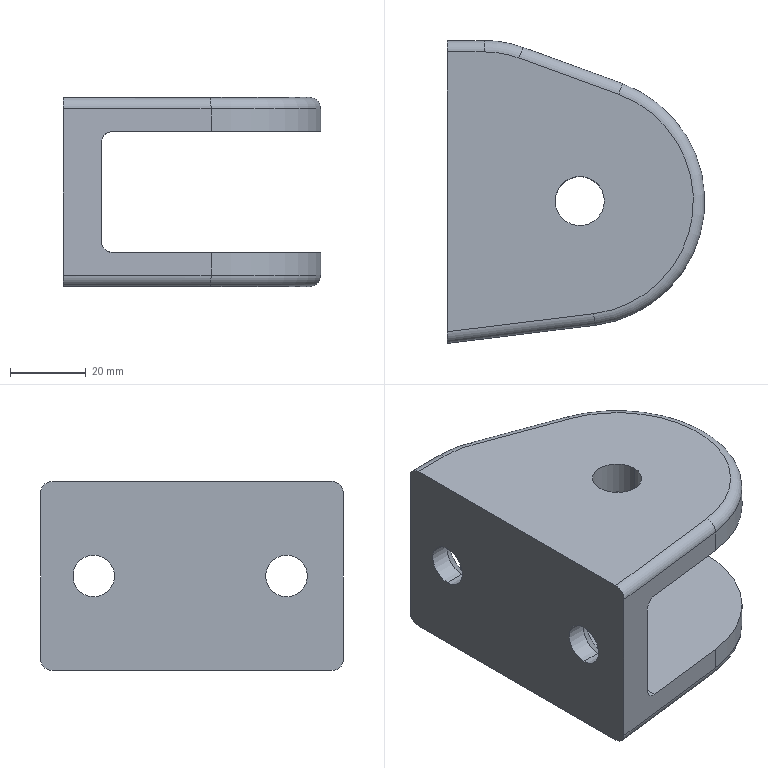Part | SolidWorks | features Fillet 2, ICE 2, Extrusion 1, HoleWzd 1 | 1 solid | 37 faces | box 68.028 x 80 x 50 mm | volume 98491 mm3 | cylinder 19 | plane 10 | cone 4 | torus 4 | commonest cylinder face diameters 6 x8 11 x4 13 x4 66.055 x2 60 x1
STEP:
#1=CARTESIAN_POINT('',(5.35,65.999,5.5));
#2=VERTEX_POINT('',#1);
#3=CARTESIAN_POINT('',(5.35,65.999,-5.5));
#4=VERTEX_POINT('',#3);
#5=CARTESIAN_POINT('',(5.35,65.999,0.));
#6=DIRECTION('',(1.,0.,0.));
#7=DIRECTION('',(0.,0.,-1.));
#8=AXIS2_PLACEMENT_3D('',#5,#6,#7);
#9=CIRCLE('',#8,5.5);
#10=EDGE_CURVE('',#2,#4,#9,.T.);
#11=ORIENTED_EDGE('',*,*,#10,.F.);
#12=CARTESIAN_POINT('',(10.,65.999,10.15));
#13=VERTEX_POINT('',#12);
#14=CARTESIAN_POINT('',(10.,65.999,10.15));
#15=DIRECTION('',(0.7071,0.,0.7071));
#16=VECTOR('',#15,1000.);
#17=LINE('',#14,#16);
#18=EDGE_CURVE('',#2,#13,#17,.T.);
#19=ORIENTED_EDGE('',*,*,#18,.T.);
#20=CARTESIAN_POINT('',(10.,65.999,-10.15));
#21=VERTEX_POINT('',#20);
#22=CARTESIAN_POINT('',(10.,65.999,0.));
#23=DIRECTION('',(1.,0.,0.));
#24=DIRECTION('',(0.,0.,-1.));
#25=AXIS2_PLACEMENT_3D('',#22,#23,#24);
#26=CIRCLE('',#25,10.15);
#27=EDGE_CURVE('',#13,#21,#26,.T.);
#28=ORIENTED_EDGE('',*,*,#27,.T.);
#29=CARTESIAN_POINT('',(10.,65.999,-10.15));
#30=DIRECTION('',(0.7071,0.,-0.7071));
#31=VECTOR('',#30,1000.);
#32=LINE('',#29,#31);
#33=EDGE_CURVE('',#4,#21,#32,.T.);
#34=ORIENTED_EDGE('',*,*,#33,.F.);
#35=EDGE_LOOP('',(#11,#19,#28,#34));
#36=FACE_OUTER_BOUND('',#35,.T.);
#37=CARTESIAN_POINT('',(10.,65.999,0.));
#38=DIRECTION('',(1.,0.,0.));
#39=DIRECTION('',(0.,0.,-1.));
#40=AXIS2_PLACEMENT_3D('',#37,#38,#39);
#41=CONICAL_SURFACE('',#40,10.15,0.7854);
#42=ADVANCED_FACE('',(#36),#41,.F.);
#43=CARTESIAN_POINT('',(0.,65.999,5.5));
#44=VERTEX_POINT('',#43);
#45=CARTESIAN_POINT('',(0.,65.999,-5.5));
#46=VERTEX_POINT('',#45);
#47=CARTESIAN_POINT('',(0.,65.999,0.));
#48=DIRECTION('',(1.,0.,0.));
#49=DIRECTION('',(0.,0.,-1.));
#50=AXIS2_PLACEMENT_3D('',#47,#48,#49);
#51=CIRCLE('',#50,5.5);
#52=EDGE_CURVE('',#44,#46,#51,.T.);
#53=ORIENTED_EDGE('',*,*,#52,.F.);
#54=CARTESIAN_POINT('',(10.,65.999,5.5));
#55=DIRECTION('',(1.,0.,0.));
#56=VECTOR('',#55,1000.);
#57=LINE('',#54,#56);
#58=EDGE_CURVE('',#44,#2,#57,.T.);
#59=ORIENTED_EDGE('',*,*,#58,.T.);
#60=ORIENTED_EDGE('',*,*,#10,.T.);
#61=CARTESIAN_POINT('',(10.,65.999,-5.5));
#62=DIRECTION('',(1.,0.,0.));
#63=VECTOR('',#62,1000.);
#64=LINE('',#61,#63);
#65=EDGE_CURVE('',#46,#4,#64,.T.);
#66=ORIENTED_EDGE('',*,*,#65,.F.);
#67=EDGE_LOOP('',(#53,#59,#60,#66));
#68=FACE_OUTER_BOUND('',#67,.T.);
#69=CARTESIAN_POINT('',(10.,65.999,0.));
#70=DIRECTION('',(1.,0.,0.));
#71=DIRECTION('',(0.,0.,-1.));
#72=AXIS2_PLACEMENT_3D('',#69,#70,#71);
#73=CYLINDRICAL_SURFACE('',#72,5.5);
#74=ADVANCED_FACE('',(#68),#73,.F.);
#75=CARTESIAN_POINT('',(5.35,15.,5.5));
#76=VERTEX_POINT('',#75);
#77=CARTESIAN_POINT('',(5.35,15.,-5.5));
#78=VERTEX_POINT('',#77);
#79=CARTESIAN_POINT('',(5.35,15.,0.));
#80=DIRECTION('',(1.,0.,0.));
#81=DIRECTION('',(0.,0.,-1.));
#82=AXIS2_PLACEMENT_3D('',#79,#80,#81);
#83=CIRCLE('',#82,5.5);
#84=EDGE_CURVE('',#76,#78,#83,.T.);
#85=ORIENTED_EDGE('',*,*,#84,.F.);
#86=CARTESIAN_POINT('',(10.,15.,10.15));
#87=VERTEX_POINT('',#86);
#88=CARTESIAN_POINT('',(10.,15.,10.15));
#89=DIRECTION('',(0.7071,0.,0.7071));
#90=VECTOR('',#89,1000.);
#91=LINE('',#88,#90);
#92=EDGE_CURVE('',#76,#87,#91,.T.);
#93=ORIENTED_EDGE('',*,*,#92,.T.);
#94=CARTESIAN_POINT('',(10.,15.,-10.15));
#95=VERTEX_POINT('',#94);
#96=CARTESIAN_POINT('',(10.,15.,0.));
#97=DIRECTION('',(1.,0.,0.));
#98=DIRECTION('',(0.,0.,-1.));
#99=AXIS2_PLACEMENT_3D('',#96,#97,#98);
#100=CIRCLE('',#99,10.15);
#101=EDGE_CURVE('',#87,#95,#100,.T.);
#102=ORIENTED_EDGE('',*,*,#101,.T.);
#103=CARTESIAN_POINT('',(10.,15.,-10.15));
#104=DIRECTION('',(0.7071,0.,-0.7071));
#105=VECTOR('',#104,1000.);
#106=LINE('',#103,#105);
#107=EDGE_CURVE('',#78,#95,#106,.T.);
#108=ORIENTED_EDGE('',*,*,#107,.F.);
#109=EDGE_LOOP('',(#85,#93,#102,#108));
#110=FACE_OUTER_BOUND('',#109,.T.);
#111=CARTESIAN_POINT('',(10.,15.,0.));
#112=DIRECTION('',(1.,0.,0.));
#113=DIRECTION('',(0.,0.,-1.));
#114=AXIS2_PLACEMENT_3D('',#111,#112,#113);
#115=CONICAL_SURFACE('',#114,10.15,0.7854);
#116=ADVANCED_FACE('',(#110),#115,.F.);
#117=CARTESIAN_POINT('',(0.,15.,5.5));
#118=VERTEX_POINT('',#117);
#119=CARTESIAN_POINT('',(0.,15.,-5.5));
#120=VERTEX_POINT('',#119);
#121=CARTESIAN_POINT('',(0.,15.,0.));
#122=DIRECTION('',(1.,0.,0.));
#123=DIRECTION('',(0.,0.,-1.));
#124=AXIS2_PLACEMENT_3D('',#121,#122,#123);
#125=CIRCLE('',#124,5.5);
#126=EDGE_CURVE('',#118,#120,#125,.T.);
#127=ORIENTED_EDGE('',*,*,#126,.F.);
#128=CARTESIAN_POINT('',(10.,15.,5.5));
#129=DIRECTION('',(1.,0.,0.));
#130=VECTOR('',#129,1000.);
#131=LINE('',#128,#130);
#132=EDGE_CURVE('',#118,#76,#131,.T.);
#133=ORIENTED_EDGE('',*,*,#132,.T.);
#134=ORIENTED_EDGE('',*,*,#84,.T.);
#135=CARTESIAN_POINT('',(10.,15.,-5.5));
#136=DIRECTION('',(1.,0.,0.));
#137=VECTOR('',#136,1000.);
#138=LINE('',#135,#137);
#139=EDGE_CURVE('',#120,#78,#138,.T.);
#140=ORIENTED_EDGE('',*,*,#139,.F.);
#141=EDGE_LOOP('',(#127,#133,#134,#140));
#142=FACE_OUTER_BOUND('',#141,.T.);
#143=CARTESIAN_POINT('',(10.,15.,0.));
#144=DIRECTION('',(1.,0.,0.));
#145=DIRECTION('',(0.,0.,-1.));
#146=AXIS2_PLACEMENT_3D('',#143,#144,#145);
#147=CYLINDRICAL_SURFACE('',#146,5.5);
#148=ADVANCED_FACE('',(#142),#147,.F.);
#149=CARTESIAN_POINT('',(28.5,37.573,-25.));
#150=VERTEX_POINT('',#149);
#151=CARTESIAN_POINT('',(41.5,37.573,-25.));
#152=VERTEX_POINT('',#151);
#153=CARTESIAN_POINT('',(35.,37.573,-25.));
#154=DIRECTION('',(0.,0.,1.));
#155=DIRECTION('',(1.,0.,0.));
#156=AXIS2_PLACEMENT_3D('',#153,#154,#155);
#157=CIRCLE('',#156,6.5);
#158=EDGE_CURVE('',#150,#152,#157,.T.);
#159=ORIENTED_EDGE('',*,*,#158,.F.);
#160=CARTESIAN_POINT('',(28.5,37.573,-16.));
#161=VERTEX_POINT('',#160);
#162=CARTESIAN_POINT('',(28.5,37.573,-25.));
#163=DIRECTION('',(0.,0.,1.));
#164=VECTOR('',#163,1000.);
#165=LINE('',#162,#164);
#166=EDGE_CURVE('',#150,#161,#165,.T.);
#167=ORIENTED_EDGE('',*,*,#166,.T.);
#168=CARTESIAN_POINT('',(41.5,37.573,-16.));
#169=VERTEX_POINT('',#168);
#170=CARTESIAN_POINT('',(35.,37.573,-16.));
#171=DIRECTION('',(0.,0.,1.));
#172=DIRECTION('',(1.,0.,0.));
#173=AXIS2_PLACEMENT_3D('',#170,#171,#172);
#174=CIRCLE('',#173,6.5);
#175=EDGE_CURVE('',#161,#169,#174,.T.);
#176=ORIENTED_EDGE('',*,*,#175,.T.);
#177=CARTESIAN_POINT('',(41.5,37.573,-25.));
#178=DIRECTION('',(0.,0.,1.));
#179=VECTOR('',#178,1000.);
#180=LINE('',#177,#179);
#181=EDGE_CURVE('',#152,#169,#180,.T.);
#182=ORIENTED_EDGE('',*,*,#181,.F.);
#183=EDGE_LOOP('',(#159,#167,#176,#182));
#184=FACE_OUTER_BOUND('',#183,.T.);
#185=CARTESIAN_POINT('',(35.,37.573,-25.));
#186=DIRECTION('',(0.,0.,1.));
#187=DIRECTION('',(1.,0.,0.));
#188=AXIS2_PLACEMENT_3D('',#185,#186,#187);
#189=CYLINDRICAL_SURFACE('',#188,6.5);
#190=ADVANCED_FACE('',(#184),#189,.F.);
#191=CARTESIAN_POINT('',(28.5,37.573,16.));
#192=VERTEX_POINT('',#191);
#193=CARTESIAN_POINT('',(41.5,37.573,16.));
#194=VERTEX_POINT('',#193);
#195=CARTESIAN_POINT('',(35.,37.573,16.));
#196=DIRECTION('',(0.,0.,1.));
#197=DIRECTION('',(1.,0.,0.));
#198=AXIS2_PLACEMENT_3D('',#195,#196,#197);
#199=CIRCLE('',#198,6.5);
#200=EDGE_CURVE('',#192,#194,#199,.T.);
#201=ORIENTED_EDGE('',*,*,#200,.F.);
#202=CARTESIAN_POINT('',(28.5,37.573,25.));
#203=VERTEX_POINT('',#202);
#204=CARTESIAN_POINT('',(28.5,37.573,-25.));
#205=DIRECTION('',(0.,0.,1.));
#206=VECTOR('',#205,1000.);
#207=LINE('',#204,#206);
#208=EDGE_CURVE('',#192,#203,#207,.T.);
#209=ORIENTED_EDGE('',*,*,#208,.T.);
#210=CARTESIAN_POINT('',(41.5,37.573,25.));
#211=VERTEX_POINT('',#210);
#212=CARTESIAN_POINT('',(35.,37.573,25.));
#213=DIRECTION('',(0.,0.,1.));
#214=DIRECTION('',(1.,0.,0.));
#215=AXIS2_PLACEMENT_3D('',#212,#213,#214);
#216=CIRCLE('',#215,6.5);
#217=EDGE_CURVE('',#203,#211,#216,.T.);
#218=ORIENTED_EDGE('',*,*,#217,.T.);
#219=CARTESIAN_POINT('',(41.5,37.573,-25.));
#220=DIRECTION('',(0.,0.,1.));
#221=VECTOR('',#220,1000.);
#222=LINE('',#219,#221);
#223=EDGE_CURVE('',#194,#211,#222,.T.);
#224=ORIENTED_EDGE('',*,*,#223,.F.);
#225=EDGE_LOOP('',(#201,#209,#218,#224));
#226=FACE_OUTER_BOUND('',#225,.T.);
#227=CARTESIAN_POINT('',(35.,37.573,-25.));
#228=DIRECTION('',(0.,0.,1.));
#229=DIRECTION('',(1.,0.,0.));
#230=AXIS2_PLACEMENT_3D('',#227,#228,#229);
#231=CYLINDRICAL_SURFACE('',#230,6.5);
#232=ADVANCED_FACE('',(#226),#231,.F.);
#233=CARTESIAN_POINT('',(0.,0.,22.));
#234=VERTEX_POINT('',#233);
#235=CARTESIAN_POINT('',(0.,0.,-22.));
#236=VERTEX_POINT('',#235);
#237=CARTESIAN_POINT('',(0.,0.,25.));
#238=DIRECTION('',(0.,0.,-1.));
#239=VECTOR('',#238,1000.);
#240=LINE('',#237,#239);
#241=EDGE_CURVE('',#234,#236,#240,.T.);
#242=ORIENTED_EDGE('',*,*,#241,.T.);
#243=CARTESIAN_POINT('',(39.025,4.792,-22.));
#244=VERTEX_POINT('',#243);
#245=CARTESIAN_POINT('',(39.025,4.792,-22.));
#246=DIRECTION('',(0.9925,0.1219,0.));
#247=VECTOR('',#246,1000.);
#248=LINE('',#245,#247);
#249=EDGE_CURVE('',#236,#244,#248,.T.);
#250=ORIENTED_EDGE('',*,*,#249,.T.);
#251=CARTESIAN_POINT('',(39.025,4.792,-16.));
#252=VERTEX_POINT('',#251);
#253=CARTESIAN_POINT('',(39.025,4.792,25.));
#254=DIRECTION('',(0.,0.,-1.));
#255=VECTOR('',#254,1000.);
#256=LINE('',#253,#255);
#257=EDGE_CURVE('',#252,#244,#256,.T.);
#258=ORIENTED_EDGE('',*,*,#257,.F.);
#259=CARTESIAN_POINT('',(13.,1.596,-16.));
#260=VERTEX_POINT('',#259);
#261=CARTESIAN_POINT('',(39.025,4.792,-16.));
#262=DIRECTION('',(0.9925,0.1219,0.));
#263=VECTOR('',#262,1000.);
#264=LINE('',#261,#263);
#265=EDGE_CURVE('',#260,#252,#264,.T.);
#266=ORIENTED_EDGE('',*,*,#265,.F.);
#267=CARTESIAN_POINT('',(10.,1.228,-13.));
#268=VERTEX_POINT('',#267);
#269=CARTESIAN_POINT('',(13.,1.596,-16.));
#270=CARTESIAN_POINT('',(11.243,1.38,-16.));
#271=CARTESIAN_POINT('',(10.,1.228,-14.757));
#272=CARTESIAN_POINT('',(10.,1.228,-13.));
#273=(BOUNDED_CURVE()B_SPLINE_CURVE(3,(#269,#270,#271,#272),.UNSPECIFIED.,.F.,.F.)B_SPLINE_CURVE_WITH_KNOTS((4,4),(4.712,6.283),.UNSPECIFIED.)CURVE()GEOMETRIC_REPRESENTATION_ITEM()RATIONAL_B_SPLINE_CURVE((1.,0.8047,0.8047,1.))REPRESENTATION_ITEM(''));
#274=EDGE_CURVE('',#260,#268,#273,.T.);
#275=ORIENTED_EDGE('',*,*,#274,.T.);
#276=CARTESIAN_POINT('',(10.,1.228,13.));
#277=VERTEX_POINT('',#276);
#278=CARTESIAN_POINT('',(10.,1.228,25.));
#279=DIRECTION('',(0.,0.,1.));
#280=VECTOR('',#279,1000.);
#281=LINE('',#278,#280);
#282=EDGE_CURVE('',#268,#277,#281,.T.);
#283=ORIENTED_EDGE('',*,*,#282,.T.);
#284=CARTESIAN_POINT('',(13.,1.596,16.));
#285=VERTEX_POINT('',#284);
#286=CARTESIAN_POINT('',(10.,1.228,13.));
#287=CARTESIAN_POINT('',(10.,1.228,14.757));
#288=CARTESIAN_POINT('',(11.243,1.38,16.));
#289=CARTESIAN_POINT('',(13.,1.596,16.));
#290=(BOUNDED_CURVE()B_SPLINE_CURVE(3,(#286,#287,#288,#289),.UNSPECIFIED.,.F.,.F.)B_SPLINE_CURVE_WITH_KNOTS((4,4),(3.142,4.712),.UNSPECIFIED.)CURVE()GEOMETRIC_REPRESENTATION_ITEM()RATIONAL_B_SPLINE_CURVE((1.,0.8047,0.8047,1.))REPRESENTATION_ITEM(''));
#291=EDGE_CURVE('',#277,#285,#290,.T.);
#292=ORIENTED_EDGE('',*,*,#291,.T.);
#293=CARTESIAN_POINT('',(39.025,4.792,16.));
#294=VERTEX_POINT('',#293);
#295=CARTESIAN_POINT('',(39.025,4.792,16.));
#296=DIRECTION('',(0.9925,0.1219,0.));
#297=VECTOR('',#296,1000.);
#298=LINE('',#295,#297);
#299=EDGE_CURVE('',#285,#294,#298,.T.);
#300=ORIENTED_EDGE('',*,*,#299,.T.);
#301=CARTESIAN_POINT('',(39.025,4.792,22.));
#302=VERTEX_POINT('',#301);
#303=CARTESIAN_POINT('',(39.025,4.792,25.));
#304=DIRECTION('',(0.,0.,-1.));
#305=VECTOR('',#304,1000.);
#306=LINE('',#303,#305);
#307=EDGE_CURVE('',#302,#294,#306,.T.);
#308=ORIENTED_EDGE('',*,*,#307,.F.);
#309=CARTESIAN_POINT('',(39.025,4.792,22.));
#310=DIRECTION('',(-0.9925,-0.1219,0.));
#311=VECTOR('',#310,1000.);
#312=LINE('',#309,#311);
#313=EDGE_CURVE('',#302,#234,#312,.T.);
#314=ORIENTED_EDGE('',*,*,#313,.T.);
#315=EDGE_LOOP('',(#242,#250,#258,#266,#275,#283,#292,#300,#308,#314));
#316=FACE_OUTER_BOUND('',#315,.T.);
#317=CARTESIAN_POINT('',(39.025,4.792,25.));
#318=DIRECTION('',(-0.1219,0.9925,0.));
#319=DIRECTION('',(-0.9925,-0.1219,0.));
#320=AXIS2_PLACEMENT_3D('',#317,#318,#319);
#321=PLANE('',#320);
#322=ADVANCED_FACE('',(#316),#321,.F.);
#323=ORIENTED_EDGE('',*,*,#257,.T.);
#324=CARTESIAN_POINT('',(46.296,68.609,-22.));
#325=VERTEX_POINT('',#324);
#326=CARTESIAN_POINT('',(35.,37.573,-22.));
#327=DIRECTION('',(0.,0.,1.));
#328=DIRECTION('',(-1.,0.,0.));
#329=AXIS2_PLACEMENT_3D('',#326,#327,#328);
#330=CIRCLE('',#329,33.028);
#331=EDGE_CURVE('',#244,#325,#330,.T.);
#332=ORIENTED_EDGE('',*,*,#331,.T.);
#333=CARTESIAN_POINT('',(46.296,68.609,-16.));
#334=VERTEX_POINT('',#333);
#335=CARTESIAN_POINT('',(46.296,68.609,25.));
#336=DIRECTION('',(0.,0.,-1.));
#337=VECTOR('',#336,1000.);
#338=LINE('',#335,#337);
#339=EDGE_CURVE('',#334,#325,#338,.T.);
#340=ORIENTED_EDGE('',*,*,#339,.F.);
#341=CARTESIAN_POINT('',(35.,37.573,-16.));
#342=DIRECTION('',(0.,0.,1.));
#343=DIRECTION('',(1.,0.,0.));
#344=AXIS2_PLACEMENT_3D('',#341,#342,#343);
#345=CIRCLE('',#344,33.028);
#346=EDGE_CURVE('',#252,#334,#345,.T.);
#347=ORIENTED_EDGE('',*,*,#346,.F.);
#348=EDGE_LOOP('',(#323,#332,#340,#347));
#349=FACE_OUTER_BOUND('',#348,.T.);
#350=CARTESIAN_POINT('',(35.,37.573,25.));
#351=DIRECTION('',(0.,0.,-1.));
#352=DIRECTION('',(-1.,0.,0.));
#353=AXIS2_PLACEMENT_3D('',#350,#351,#352);
#354=CYLINDRICAL_SURFACE('',#353,33.028);
#355=ADVANCED_FACE('',(#349),#354,.T.);
#356=ORIENTED_EDGE('',*,*,#339,.T.);
#357=CARTESIAN_POINT('',(19.971,78.191,-22.));
#358=VERTEX_POINT('',#357);
#359=CARTESIAN_POINT('',(19.971,78.191,-22.));
#360=DIRECTION('',(-0.9397,0.342,0.));
#361=VECTOR('',#360,1000.);
#362=LINE('',#359,#361);
#363=EDGE_CURVE('',#325,#358,#362,.T.);
#364=ORIENTED_EDGE('',*,*,#363,.T.);
#365=CARTESIAN_POINT('',(19.971,78.191,-16.));
#366=VERTEX_POINT('',#365);
#367=CARTESIAN_POINT('',(19.971,78.191,25.));
#368=DIRECTION('',(0.,0.,-1.));
#369=VECTOR('',#368,1000.);
#370=LINE('',#367,#369);
#371=EDGE_CURVE('',#366,#358,#370,.T.);
#372=ORIENTED_EDGE('',*,*,#371,.F.);
#373=CARTESIAN_POINT('',(19.971,78.191,-16.));
#374=DIRECTION('',(-0.9397,0.342,0.));
#375=VECTOR('',#374,1000.);
#376=LINE('',#373,#375);
#377=EDGE_CURVE('',#334,#366,#376,.T.);
#378=ORIENTED_EDGE('',*,*,#377,.F.);
#379=EDGE_LOOP('',(#356,#364,#372,#378));
#380=FACE_OUTER_BOUND('',#379,.T.);
#381=CARTESIAN_POINT('',(19.971,78.191,25.));
#382=DIRECTION('',(-0.342,-0.9397,0.));
#383=DIRECTION('',(0.9397,-0.342,0.));
#384=AXIS2_PLACEMENT_3D('',#381,#382,#383);
#385=PLANE('',#384);
#386=ADVANCED_FACE('',(#380),#385,.F.);
#387=ORIENTED_EDGE('',*,*,#371,.T.);
#388=CARTESIAN_POINT('',(9.71,80.,-22.));
#389=VERTEX_POINT('',#388);
#390=CARTESIAN_POINT('',(9.71,50.,-22.));
#391=DIRECTION('',(0.,0.,1.));
#392=DIRECTION('',(-1.,0.,0.));
#393=AXIS2_PLACEMENT_3D('',#390,#391,#392);
#394=CIRCLE('',#393,30.);
#395=EDGE_CURVE('',#358,#389,#394,.T.);
#396=ORIENTED_EDGE('',*,*,#395,.T.);
#397=CARTESIAN_POINT('',(9.71,80.,22.));
#398=VERTEX_POINT('',#397);
#399=CARTESIAN_POINT('',(9.71,80.,25.));
#400=DIRECTION('',(0.,0.,-1.));
#401=VECTOR('',#400,1000.);
#402=LINE('',#399,#401);
#403=EDGE_CURVE('',#398,#389,#402,.T.);
#404=ORIENTED_EDGE('',*,*,#403,.F.);
#405=CARTESIAN_POINT('',(19.971,78.191,22.));
#406=VERTEX_POINT('',#405);
#407=CARTESIAN_POINT('',(9.71,50.,22.));
#408=DIRECTION('',(0.,0.,-1.));
#409=DIRECTION('',(-1.,0.,0.));
#410=AXIS2_PLACEMENT_3D('',#407,#408,#409);
#411=CIRCLE('',#410,30.);
#412=EDGE_CURVE('',#398,#406,#411,.T.);
#413=ORIENTED_EDGE('',*,*,#412,.T.);
#414=CARTESIAN_POINT('',(19.971,78.191,16.));
#415=VERTEX_POINT('',#414);
#416=CARTESIAN_POINT('',(19.971,78.191,25.));
#417=DIRECTION('',(0.,0.,-1.));
#418=VECTOR('',#417,1000.);
#419=LINE('',#416,#418);
#420=EDGE_CURVE('',#406,#415,#419,.T.);
#421=ORIENTED_EDGE('',*,*,#420,.T.);
#422=CARTESIAN_POINT('',(13.,79.819,16.));
#423=VERTEX_POINT('',#422);
#424=CARTESIAN_POINT('',(9.71,50.,16.));
#425=DIRECTION('',(0.,0.,1.));
#426=DIRECTION('',(1.,0.,0.));
#427=AXIS2_PLACEMENT_3D('',#424,#425,#426);
#428=CIRCLE('',#427,30.);
#429=EDGE_CURVE('',#415,#423,#428,.T.);
#430=ORIENTED_EDGE('',*,*,#429,.T.);
#431=CARTESIAN_POINT('',(10.,79.999,13.));
#432=VERTEX_POINT('',#431);
#433=CARTESIAN_POINT('',(13.,79.819,16.));
#434=CARTESIAN_POINT('',(12.803,79.841,16.));
#435=CARTESIAN_POINT('',(12.609,79.86,15.981));
#436=CARTESIAN_POINT('',(12.227,79.895,15.905));
#437=CARTESIAN_POINT('',(12.036,79.91,15.848));
#438=CARTESIAN_POINT('',(11.673,79.936,15.698));
#439=CARTESIAN_POINT('',(11.501,79.947,15.606));
#440=CARTESIAN_POINT('',(11.175,79.965,15.389));
#441=CARTESIAN_POINT('',(11.02,79.972,15.262));
#442=CARTESIAN_POINT('',(10.743,79.983,14.986));
#443=CARTESIAN_POINT('',(10.618,79.986,14.835));
#444=CARTESIAN_POINT('',(10.399,79.992,14.507));
#445=CARTESIAN_POINT('',(10.305,79.994,14.332));
#446=CARTESIAN_POINT('',(10.155,79.997,13.971));
#447=CARTESIAN_POINT('',(10.097,79.998,13.782));
#448=CARTESIAN_POINT('',(10.019,79.998,13.394));
#449=CARTESIAN_POINT('',(10.,79.999,13.198));
#450=CARTESIAN_POINT('',(10.,79.999,13.));
#451=B_SPLINE_CURVE_WITH_KNOTS('',3,(#433,#434,#435,#436,#437,#438,#439,#440,#441,#442,#443,#444,#445,#446,#447,#448,#449,#450),.UNSPECIFIED.,.F.,.F.,(4,2,2,2,2,2,2,2,4),(0.,0.0005866,0.001173,0.00176,0.002346,0.002933,0.00352,0.004106,0.004693),.UNSPECIFIED.);
#452=EDGE_CURVE('',#423,#432,#451,.T.);
#453=ORIENTED_EDGE('',*,*,#452,.T.);
#454=CARTESIAN_POINT('',(10.,79.999,-13.));
#455=VERTEX_POINT('',#454);
#456=CARTESIAN_POINT('',(10.,79.999,25.));
#457=DIRECTION('',(0.,0.,-1.));
#458=VECTOR('',#457,1000.);
#459=LINE('',#456,#458);
#460=EDGE_CURVE('',#432,#455,#459,.T.);
#461=ORIENTED_EDGE('',*,*,#460,.T.);
#462=CARTESIAN_POINT('',(13.,79.819,-16.));
#463=VERTEX_POINT('',#462);
#464=CARTESIAN_POINT('',(10.,79.999,-13.));
#465=CARTESIAN_POINT('',(10.,79.999,-13.198));
#466=CARTESIAN_POINT('',(10.019,79.998,-13.393));
#467=CARTESIAN_POINT('',(10.096,79.998,-13.777));
#468=CARTESIAN_POINT('',(10.154,79.997,-13.968));
#469=CARTESIAN_POINT('',(10.304,79.994,-14.331));
#470=CARTESIAN_POINT('',(10.397,79.992,-14.504));
#471=CARTESIAN_POINT('',(10.615,79.987,-14.83));
#472=CARTESIAN_POINT('',(10.741,79.983,-14.984));
#473=CARTESIAN_POINT('',(11.018,79.972,-15.261));
#474=CARTESIAN_POINT('',(11.17,79.965,-15.385));
#475=CARTESIAN_POINT('',(11.498,79.947,-15.604));
#476=CARTESIAN_POINT('',(11.672,79.936,-15.697));
#477=CARTESIAN_POINT('',(12.033,79.911,-15.846));
#478=CARTESIAN_POINT('',(12.221,79.895,-15.904));
#479=CARTESIAN_POINT('',(12.608,79.86,-15.981));
#480=CARTESIAN_POINT('',(12.803,79.841,-16.));
#481=CARTESIAN_POINT('',(13.,79.819,-16.));
#482=B_SPLINE_CURVE_WITH_KNOTS('',3,(#464,#465,#466,#467,#468,#469,#470,#471,#472,#473,#474,#475,#476,#477,#478,#479,#480,#481),.UNSPECIFIED.,.F.,.F.,(4,2,2,2,2,2,2,2,4),(0.,0.0005866,0.001173,0.00176,0.002346,0.002933,0.003519,0.004106,0.004693),.UNSPECIFIED.);
#483=EDGE_CURVE('',#455,#463,#482,.T.);
#484=ORIENTED_EDGE('',*,*,#483,.T.);
#485=CARTESIAN_POINT('',(9.71,50.,-16.));
#486=DIRECTION('',(0.,0.,1.));
#487=DIRECTION('',(1.,0.,0.));
#488=AXIS2_PLACEMENT_3D('',#485,#486,#487);
#489=CIRCLE('',#488,30.);
#490=EDGE_CURVE('',#366,#463,#489,.T.);
#491=ORIENTED_EDGE('',*,*,#490,.F.);
#492=EDGE_LOOP('',(#387,#396,#404,#413,#421,#430,#453,#461,#484,#491));
#493=FACE_OUTER_BOUND('',#492,.T.);
#494=CARTESIAN_POINT('',(9.71,50.,25.));
#495=DIRECTION('',(0.,0.,-1.));
#496=DIRECTION('',(-1.,0.,0.));
#497=AXIS2_PLACEMENT_3D('',#494,#495,#496);
#498=CYLINDRICAL_SURFACE('',#497,30.);
#499=ADVANCED_FACE('',(#493),#498,.T.);
#500=CARTESIAN_POINT('',(46.296,68.609,22.));
#501=VERTEX_POINT('',#500);
#502=CARTESIAN_POINT('',(46.296,68.609,16.));
#503=VERTEX_POINT('',#502);
#504=CARTESIAN_POINT('',(46.296,68.609,25.));
#505=DIRECTION('',(0.,0.,-1.));
#506=VECTOR('',#505,1000.);
#507=LINE('',#504,#506);
#508=EDGE_CURVE('',#501,#503,#507,.T.);
#509=ORIENTED_EDGE('',*,*,#508,.F.);
#510=CARTESIAN_POINT('',(35.,37.573,22.));
#511=DIRECTION('',(0.,0.,-1.));
#512=DIRECTION('',(-1.,0.,0.));
#513=AXIS2_PLACEMENT_3D('',#510,#511,#512);
#514=CIRCLE('',#513,33.028);
#515=EDGE_CURVE('',#501,#302,#514,.T.);
#516=ORIENTED_EDGE('',*,*,#515,.T.);
#517=ORIENTED_EDGE('',*,*,#307,.T.);
#518=CARTESIAN_POINT('',(35.,37.573,16.));
#519=DIRECTION('',(0.,0.,1.));
#520=DIRECTION('',(1.,0.,0.));
#521=AXIS2_PLACEMENT_3D('',#518,#519,#520);
#522=CIRCLE('',#521,33.028);
#523=EDGE_CURVE('',#294,#503,#522,.T.);
#524=ORIENTED_EDGE('',*,*,#523,.T.);
#525=EDGE_LOOP('',(#509,#516,#517,#524));
#526=FACE_OUTER_BOUND('',#525,.T.);
#527=CARTESIAN_POINT('',(35.,37.573,25.));
#528=DIRECTION('',(0.,0.,-1.));
#529=DIRECTION('',(-1.,0.,0.));
#530=AXIS2_PLACEMENT_3D('',#527,#528,#529);
#531=CYLINDRICAL_SURFACE('',#530,33.028);
#532=ADVANCED_FACE('',(#526),#531,.T.);
#533=ORIENTED_EDGE('',*,*,#420,.F.);
#534=CARTESIAN_POINT('',(19.971,78.191,22.));
#535=DIRECTION('',(0.9397,-0.342,0.));
#536=VECTOR('',#535,1000.);
#537=LINE('',#534,#536);
#538=EDGE_CURVE('',#406,#501,#537,.T.);
#539=ORIENTED_EDGE('',*,*,#538,.T.);
#540=ORIENTED_EDGE('',*,*,#508,.T.);
#541=CARTESIAN_POINT('',(19.971,78.191,16.));
#542=DIRECTION('',(-0.9397,0.342,0.));
#543=VECTOR('',#542,1000.);
#544=LINE('',#541,#543);
#545=EDGE_CURVE('',#503,#415,#544,.T.);
#546=ORIENTED_EDGE('',*,*,#545,.T.);
#547=EDGE_LOOP('',(#533,#539,#540,#546));
#548=FACE_OUTER_BOUND('',#547,.T.);
#549=CARTESIAN_POINT('',(19.971,78.191,25.));
#550=DIRECTION('',(-0.342,-0.9397,0.));
#551=DIRECTION('',(0.9397,-0.342,0.));
#552=AXIS2_PLACEMENT_3D('',#549,#550,#551);
#553=PLANE('',#552);
#554=ADVANCED_FACE('',(#548),#553,.F.);
#555=ORIENTED_EDGE('',*,*,#403,.T.);
#556=CARTESIAN_POINT('',(0.,80.,-22.));
#557=VERTEX_POINT('',#556);
#558=CARTESIAN_POINT('',(0.,80.,-22.));
#559=DIRECTION('',(-1.,0.,0.));
#560=VECTOR('',#559,1000.);
#561=LINE('',#558,#560);
#562=EDGE_CURVE('',#389,#557,#561,.T.);
#563=ORIENTED_EDGE('',*,*,#562,.T.);
#564=CARTESIAN_POINT('',(0.,80.,22.));
#565=VERTEX_POINT('',#564);
#566=CARTESIAN_POINT('',(0.,80.,25.));
#567=DIRECTION('',(0.,0.,-1.));
#568=VECTOR('',#567,1000.);
#569=LINE('',#566,#568);
#570=EDGE_CURVE('',#565,#557,#569,.T.);
#571=ORIENTED_EDGE('',*,*,#570,.F.);
#572=CARTESIAN_POINT('',(0.,80.,22.));
#573=DIRECTION('',(1.,0.,0.));
#574=VECTOR('',#573,1000.);
#575=LINE('',#572,#574);
#576=EDGE_CURVE('',#565,#398,#575,.T.);
#577=ORIENTED_EDGE('',*,*,#576,.T.);
#578=EDGE_LOOP('',(#555,#563,#571,#577));
#579=FACE_OUTER_BOUND('',#578,.T.);
#580=CARTESIAN_POINT('',(0.,80.,25.));
#581=DIRECTION('',(0.,-1.,0.));
#582=DIRECTION('',(0.,0.,-1.));
#583=AXIS2_PLACEMENT_3D('',#580,#581,#582);
#584=PLANE('',#583);
#585=ADVANCED_FACE('',(#579),#584,.F.);
#586=CARTESIAN_POINT('',(0.,65.999,0.));
#587=DIRECTION('',(1.,0.,0.));
#588=DIRECTION('',(0.,0.,-1.));
#589=AXIS2_PLACEMENT_3D('',#586,#587,#588);
#590=CIRCLE('',#589,5.5);
#591=EDGE_CURVE('',#46,#44,#590,.T.);
#592=ORIENTED_EDGE('',*,*,#591,.T.);
#593=ORIENTED_EDGE('',*,*,#52,.T.);
#594=EDGE_LOOP('',(#592,#593));
#595=FACE_BOUND('',#594,.T.);
#596=CARTESIAN_POINT('',(0.,15.,0.));
#597=DIRECTION('',(1.,0.,0.));
#598=DIRECTION('',(0.,0.,-1.));
#599=AXIS2_PLACEMENT_3D('',#596,#597,#598);
#600=CIRCLE('',#599,5.5);
#601=EDGE_CURVE('',#120,#118,#600,.T.);
#602=ORIENTED_EDGE('',*,*,#601,.T.);
#603=ORIENTED_EDGE('',*,*,#126,.T.);
#604=EDGE_LOOP('',(#602,#603));
#605=FACE_BOUND('',#604,.T.);
#606=CARTESIAN_POINT('',(0.,77.,-25.));
#607=VERTEX_POINT('',#606);
#608=CARTESIAN_POINT('',(0.,3.023,-25.));
#609=VERTEX_POINT('',#608);
#610=CARTESIAN_POINT('',(0.,0.,-25.));
#611=DIRECTION('',(0.,-1.,0.));
#612=VECTOR('',#611,1000.);
#613=LINE('',#610,#612);
#614=EDGE_CURVE('',#607,#609,#613,.T.);
#615=ORIENTED_EDGE('',*,*,#614,.T.);
#616=CARTESIAN_POINT('',(0.,3.023,-25.));
#617=CARTESIAN_POINT('',(0.,1.252,-25.));
#618=CARTESIAN_POINT('',(0.,0.,-23.757));
#619=CARTESIAN_POINT('',(0.,0.,-22.));
#620=(BOUNDED_CURVE()B_SPLINE_CURVE(3,(#616,#617,#618,#619),.UNSPECIFIED.,.F.,.F.)B_SPLINE_CURVE_WITH_KNOTS((4,4),(4.712,6.283),.UNSPECIFIED.)CURVE()GEOMETRIC_REPRESENTATION_ITEM()RATIONAL_B_SPLINE_CURVE((1.,0.8047,0.8047,1.))REPRESENTATION_ITEM(''));
#621=EDGE_CURVE('',#609,#236,#620,.T.);
#622=ORIENTED_EDGE('',*,*,#621,.T.);
#623=ORIENTED_EDGE('',*,*,#241,.F.);
#624=CARTESIAN_POINT('',(0.,3.023,25.));
#625=VERTEX_POINT('',#624);
#626=CARTESIAN_POINT('',(0.,0.,22.));
#627=CARTESIAN_POINT('',(0.,0.,23.757));
#628=CARTESIAN_POINT('',(0.,1.252,25.));
#629=CARTESIAN_POINT('',(0.,3.023,25.));
#630=(BOUNDED_CURVE()B_SPLINE_CURVE(3,(#626,#627,#628,#629),.UNSPECIFIED.,.F.,.F.)B_SPLINE_CURVE_WITH_KNOTS((4,4),(3.142,4.712),.UNSPECIFIED.)CURVE()GEOMETRIC_REPRESENTATION_ITEM()RATIONAL_B_SPLINE_CURVE((1.,0.8047,0.8047,1.))REPRESENTATION_ITEM(''));
#631=EDGE_CURVE('',#234,#625,#630,.T.);
#632=ORIENTED_EDGE('',*,*,#631,.T.);
#633=CARTESIAN_POINT('',(0.,77.,25.));
#634=VERTEX_POINT('',#633);
#635=CARTESIAN_POINT('',(0.,0.,25.));
#636=DIRECTION('',(0.,-1.,0.));
#637=VECTOR('',#636,1000.);
#638=LINE('',#635,#637);
#639=EDGE_CURVE('',#634,#625,#638,.T.);
#640=ORIENTED_EDGE('',*,*,#639,.F.);
#641=CARTESIAN_POINT('',(0.,77.,22.));
#642=DIRECTION('',(-1.,0.,0.));
#643=DIRECTION('',(0.,0.,-1.));
#644=AXIS2_PLACEMENT_3D('',#641,#642,#643);
#645=CIRCLE('',#644,3.);
#646=EDGE_CURVE('',#634,#565,#645,.T.);
#647=ORIENTED_EDGE('',*,*,#646,.T.);
#648=ORIENTED_EDGE('',*,*,#570,.T.);
#649=CARTESIAN_POINT('',(0.,77.,-22.));
#650=DIRECTION('',(-1.,0.,0.));
#651=DIRECTION('',(0.,0.,-1.));
#652=AXIS2_PLACEMENT_3D('',#649,#650,#651);
#653=CIRCLE('',#652,3.);
#654=EDGE_CURVE('',#557,#607,#653,.T.);
#655=ORIENTED_EDGE('',*,*,#654,.T.);
#656=EDGE_LOOP('',(#615,#622,#623,#632,#640,#647,#648,#655));
#657=FACE_OUTER_BOUND('',#656,.T.);
#658=CARTESIAN_POINT('',(0.,0.,25.));
#659=DIRECTION('',(1.,0.,0.));
#660=DIRECTION('',(0.,0.,-1.));
#661=AXIS2_PLACEMENT_3D('',#658,#659,#660);
#662=PLANE('',#661);
#663=ADVANCED_FACE('',(#595,#605,#657),#662,.F.);
#664=CARTESIAN_POINT('',(35.,37.573,25.));
#665=DIRECTION('',(0.,0.,1.));
#666=DIRECTION('',(1.,0.,0.));
#667=AXIS2_PLACEMENT_3D('',#664,#665,#666);
#668=CIRCLE('',#667,6.5);
#669=EDGE_CURVE('',#211,#203,#668,.T.);
#670=ORIENTED_EDGE('',*,*,#669,.F.);
#671=ORIENTED_EDGE('',*,*,#217,.F.);
#672=EDGE_LOOP('',(#670,#671));
#673=FACE_BOUND('',#672,.T.);
#674=CARTESIAN_POINT('',(18.945,75.372,25.));
#675=VERTEX_POINT('',#674);
#676=CARTESIAN_POINT('',(9.71,77.,25.));
#677=VERTEX_POINT('',#676);
#678=CARTESIAN_POINT('',(9.71,50.,25.));
#679=DIRECTION('',(0.,0.,1.));
#680=DIRECTION('',(-1.,0.,0.));
#681=AXIS2_PLACEMENT_3D('',#678,#679,#680);
#682=CIRCLE('',#681,27.);
#683=EDGE_CURVE('',#675,#677,#682,.T.);
#684=ORIENTED_EDGE('',*,*,#683,.T.);
#685=CARTESIAN_POINT('',(9.71,77.,25.));
#686=DIRECTION('',(-1.,0.,0.));
#687=VECTOR('',#686,1000.);
#688=LINE('',#685,#687);
#689=EDGE_CURVE('',#677,#634,#688,.T.);
#690=ORIENTED_EDGE('',*,*,#689,.T.);
#691=ORIENTED_EDGE('',*,*,#639,.T.);
#692=CARTESIAN_POINT('',(38.659,7.769,25.));
#693=VERTEX_POINT('',#692);
#694=CARTESIAN_POINT('',(15.248,4.895,25.));
#695=DIRECTION('',(0.9925,0.1219,0.));
#696=VECTOR('',#695,1000.);
#697=LINE('',#694,#696);
#698=EDGE_CURVE('',#625,#693,#697,.T.);
#699=ORIENTED_EDGE('',*,*,#698,.T.);
#700=CARTESIAN_POINT('',(45.27,65.79,25.));
#701=VERTEX_POINT('',#700);
#702=CARTESIAN_POINT('',(35.,37.573,25.));
#703=DIRECTION('',(0.,0.,1.));
#704=DIRECTION('',(-1.,0.,0.));
#705=AXIS2_PLACEMENT_3D('',#702,#703,#704);
#706=CIRCLE('',#705,30.028);
#707=EDGE_CURVE('',#693,#701,#706,.T.);
#708=ORIENTED_EDGE('',*,*,#707,.T.);
#709=CARTESIAN_POINT('',(18.945,75.372,25.));
#710=DIRECTION('',(-0.9397,0.342,0.));
#711=VECTOR('',#710,1000.);
#712=LINE('',#709,#711);
#713=EDGE_CURVE('',#701,#675,#712,.T.);
#714=ORIENTED_EDGE('',*,*,#713,.T.);
#715=EDGE_LOOP('',(#684,#690,#691,#699,#708,#714));
#716=FACE_OUTER_BOUND('',#715,.T.);
#717=CARTESIAN_POINT('',(9.71,50.,25.));
#718=DIRECTION('',(0.,0.,-1.));
#719=DIRECTION('',(-1.,0.,0.));
#720=AXIS2_PLACEMENT_3D('',#717,#718,#719);
#721=PLANE('',#720);
#722=ADVANCED_FACE('',(#673,#716),#721,.F.);
#723=ORIENTED_EDGE('',*,*,#614,.F.);
#724=CARTESIAN_POINT('',(9.71,77.,-25.));
#725=VERTEX_POINT('',#724);
#726=CARTESIAN_POINT('',(9.71,77.,-25.));
#727=DIRECTION('',(1.,0.,0.));
#728=VECTOR('',#727,1000.);
#729=LINE('',#726,#728);
#730=EDGE_CURVE('',#607,#725,#729,.T.);
#731=ORIENTED_EDGE('',*,*,#730,.T.);
#732=CARTESIAN_POINT('',(18.945,75.372,-25.));
#733=VERTEX_POINT('',#732);
#734=CARTESIAN_POINT('',(9.71,50.,-25.));
#735=DIRECTION('',(0.,0.,-1.));
#736=DIRECTION('',(-1.,0.,0.));
#737=AXIS2_PLACEMENT_3D('',#734,#735,#736);
#738=CIRCLE('',#737,27.);
#739=EDGE_CURVE('',#725,#733,#738,.T.);
#740=ORIENTED_EDGE('',*,*,#739,.T.);
#741=CARTESIAN_POINT('',(45.27,65.79,-25.));
#742=VERTEX_POINT('',#741);
#743=CARTESIAN_POINT('',(45.27,65.79,-25.));
#744=DIRECTION('',(0.9397,-0.342,0.));
#745=VECTOR('',#744,1000.);
#746=LINE('',#743,#745);
#747=EDGE_CURVE('',#733,#742,#746,.T.);
#748=ORIENTED_EDGE('',*,*,#747,.T.);
#749=CARTESIAN_POINT('',(38.659,7.769,-25.));
#750=VERTEX_POINT('',#749);
#751=CARTESIAN_POINT('',(35.,37.573,-25.));
#752=DIRECTION('',(0.,0.,-1.));
#753=DIRECTION('',(-1.,0.,0.));
#754=AXIS2_PLACEMENT_3D('',#751,#752,#753);
#755=CIRCLE('',#754,30.028);
#756=EDGE_CURVE('',#742,#750,#755,.T.);
#757=ORIENTED_EDGE('',*,*,#756,.T.);
#758=CARTESIAN_POINT('',(-0.3656,2.978,-25.));
#759=DIRECTION('',(-0.9925,-0.1219,0.));
#760=VECTOR('',#759,1000.);
#761=LINE('',#758,#760);
#762=EDGE_CURVE('',#750,#609,#761,.T.);
#763=ORIENTED_EDGE('',*,*,#762,.T.);
#764=EDGE_LOOP('',(#723,#731,#740,#748,#757,#763));
#765=FACE_OUTER_BOUND('',#764,.T.);
#766=CARTESIAN_POINT('',(35.,37.573,-25.));
#767=DIRECTION('',(0.,0.,1.));
#768=DIRECTION('',(1.,0.,0.));
#769=AXIS2_PLACEMENT_3D('',#766,#767,#768);
#770=CIRCLE('',#769,6.5);
#771=EDGE_CURVE('',#152,#150,#770,.T.);
#772=ORIENTED_EDGE('',*,*,#771,.T.);
#773=ORIENTED_EDGE('',*,*,#158,.T.);
#774=EDGE_LOOP('',(#772,#773));
#775=FACE_BOUND('',#774,.T.);
#776=CARTESIAN_POINT('',(9.71,50.,-25.));
#777=DIRECTION('',(0.,0.,-1.));
#778=DIRECTION('',(-1.,0.,0.));
#779=AXIS2_PLACEMENT_3D('',#776,#777,#778);
#780=PLANE('',#779);
#781=ADVANCED_FACE('',(#765,#775),#780,.T.);
#782=CARTESIAN_POINT('',(10.,65.999,0.));
#783=DIRECTION('',(1.,0.,0.));
#784=DIRECTION('',(0.,0.,-1.));
#785=AXIS2_PLACEMENT_3D('',#782,#783,#784);
#786=CIRCLE('',#785,10.15);
#787=EDGE_CURVE('',#21,#13,#786,.T.);
#788=ORIENTED_EDGE('',*,*,#787,.F.);
#789=ORIENTED_EDGE('',*,*,#27,.F.);
#790=EDGE_LOOP('',(#788,#789));
#791=FACE_BOUND('',#790,.T.);
#792=CARTESIAN_POINT('',(10.,15.,0.));
#793=DIRECTION('',(1.,0.,0.));
#794=DIRECTION('',(0.,0.,-1.));
#795=AXIS2_PLACEMENT_3D('',#792,#793,#794);
#796=CIRCLE('',#795,10.15);
#797=EDGE_CURVE('',#95,#87,#796,.T.);
#798=ORIENTED_EDGE('',*,*,#797,.F.);
#799=ORIENTED_EDGE('',*,*,#101,.F.);
#800=EDGE_LOOP('',(#798,#799));
#801=FACE_BOUND('',#800,.T.);
#802=ORIENTED_EDGE('',*,*,#282,.F.);
#803=CARTESIAN_POINT('',(10.,90.134,-13.));
#804=DIRECTION('',(0.,1.,0.));
#805=VECTOR('',#804,1000.);
#806=LINE('',#803,#805);
#807=EDGE_CURVE('',#268,#455,#806,.T.);
#808=ORIENTED_EDGE('',*,*,#807,.T.);
#809=ORIENTED_EDGE('',*,*,#460,.F.);
#810=CARTESIAN_POINT('',(10.,1.228,13.));
#811=DIRECTION('',(0.,-1.,0.));
#812=VECTOR('',#811,1000.);
#813=LINE('',#810,#812);
#814=EDGE_CURVE('',#432,#277,#813,.T.);
#815=ORIENTED_EDGE('',*,*,#814,.T.);
#816=EDGE_LOOP('',(#802,#808,#809,#815));
#817=FACE_OUTER_BOUND('',#816,.T.);
#818=CARTESIAN_POINT('',(10.,90.134,-16.));
#819=DIRECTION('',(-1.,0.,0.));
#820=DIRECTION('',(0.,-1.,0.));
#821=AXIS2_PLACEMENT_3D('',#818,#819,#820);
#822=PLANE('',#821);
#823=ADVANCED_FACE('',(#791,#801,#817),#822,.F.);
#824=CARTESIAN_POINT('',(35.,37.573,-16.));
#825=DIRECTION('',(0.,0.,1.));
#826=DIRECTION('',(1.,0.,0.));
#827=AXIS2_PLACEMENT_3D('',#824,#825,#826);
#828=CIRCLE('',#827,6.5);
#829=EDGE_CURVE('',#169,#161,#828,.T.);
#830=ORIENTED_EDGE('',*,*,#829,.F.);
#831=ORIENTED_EDGE('',*,*,#175,.F.);
#832=EDGE_LOOP('',(#830,#831));
#833=FACE_BOUND('',#832,.T.);
#834=ORIENTED_EDGE('',*,*,#490,.T.);
#835=CARTESIAN_POINT('',(13.,0.,-16.));
#836=DIRECTION('',(0.,-1.,0.));
#837=VECTOR('',#836,1000.);
#838=LINE('',#835,#837);
#839=EDGE_CURVE('',#463,#260,#838,.T.);
#840=ORIENTED_EDGE('',*,*,#839,.T.);
#841=ORIENTED_EDGE('',*,*,#265,.T.);
#842=ORIENTED_EDGE('',*,*,#346,.T.);
#843=ORIENTED_EDGE('',*,*,#377,.T.);
#844=EDGE_LOOP('',(#834,#840,#841,#842,#843));
#845=FACE_OUTER_BOUND('',#844,.T.);
#846=CARTESIAN_POINT('',(0.,0.,-16.));
#847=DIRECTION('',(0.,0.,1.));
#848=DIRECTION('',(1.,0.,0.));
#849=AXIS2_PLACEMENT_3D('',#846,#847,#848);
#850=PLANE('',#849);
#851=ADVANCED_FACE('',(#833,#845),#850,.T.);
#852=CARTESIAN_POINT('',(35.,37.573,16.));
#853=DIRECTION('',(0.,0.,1.));
#854=DIRECTION('',(1.,0.,0.));
#855=AXIS2_PLACEMENT_3D('',#852,#853,#854);
#856=CIRCLE('',#855,6.5);
#857=EDGE_CURVE('',#194,#192,#856,.T.);
#858=ORIENTED_EDGE('',*,*,#857,.T.);
#859=ORIENTED_EDGE('',*,*,#200,.T.);
#860=EDGE_LOOP('',(#858,#859));
#861=FACE_BOUND('',#860,.T.);
#862=ORIENTED_EDGE('',*,*,#299,.F.);
#863=CARTESIAN_POINT('',(13.,79.999,16.));
#864=DIRECTION('',(0.,1.,0.));
#865=VECTOR('',#864,1000.);
#866=LINE('',#863,#865);
#867=EDGE_CURVE('',#285,#423,#866,.T.);
#868=ORIENTED_EDGE('',*,*,#867,.T.);
#869=ORIENTED_EDGE('',*,*,#429,.F.);
#870=ORIENTED_EDGE('',*,*,#545,.F.);
#871=ORIENTED_EDGE('',*,*,#523,.F.);
#872=EDGE_LOOP('',(#862,#868,#869,#870,#871));
#873=FACE_OUTER_BOUND('',#872,.T.);
#874=CARTESIAN_POINT('',(0.,0.,16.));
#875=DIRECTION('',(0.,0.,1.));
#876=DIRECTION('',(1.,0.,0.));
#877=AXIS2_PLACEMENT_3D('',#874,#875,#876);
#878=PLANE('',#877);
#879=ADVANCED_FACE('',(#861,#873),#878,.F.);
#880=ORIENTED_EDGE('',*,*,#208,.F.);
#881=ORIENTED_EDGE('',*,*,#857,.F.);
#882=ORIENTED_EDGE('',*,*,#223,.T.);
#883=ORIENTED_EDGE('',*,*,#669,.T.);
#884=EDGE_LOOP('',(#880,#881,#882,#883));
#885=FACE_OUTER_BOUND('',#884,.T.);
#886=CARTESIAN_POINT('',(35.,37.573,-25.));
#887=DIRECTION('',(0.,0.,1.));
#888=DIRECTION('',(1.,0.,0.));
#889=AXIS2_PLACEMENT_3D('',#886,#887,#888);
#890=CYLINDRICAL_SURFACE('',#889,6.5);
#891=ADVANCED_FACE('',(#885),#890,.F.);
#892=ORIENTED_EDGE('',*,*,#166,.F.);
#893=ORIENTED_EDGE('',*,*,#771,.F.);
#894=ORIENTED_EDGE('',*,*,#181,.T.);
#895=ORIENTED_EDGE('',*,*,#829,.T.);
#896=EDGE_LOOP('',(#892,#893,#894,#895));
#897=FACE_OUTER_BOUND('',#896,.T.);
#898=CARTESIAN_POINT('',(35.,37.573,-25.));
#899=DIRECTION('',(0.,0.,1.));
#900=DIRECTION('',(1.,0.,0.));
#901=AXIS2_PLACEMENT_3D('',#898,#899,#900);
#902=CYLINDRICAL_SURFACE('',#901,6.5);
#903=ADVANCED_FACE('',(#897),#902,.F.);
#904=ORIENTED_EDGE('',*,*,#654,.F.);
#905=ORIENTED_EDGE('',*,*,#562,.F.);
#906=CARTESIAN_POINT('',(9.71,77.,-22.));
#907=DIRECTION('',(1.,0.,0.));
#908=DIRECTION('',(0.,1.,0.));
#909=AXIS2_PLACEMENT_3D('',#906,#907,#908);
#910=CIRCLE('',#909,3.);
#911=EDGE_CURVE('',#725,#389,#910,.T.);
#912=ORIENTED_EDGE('',*,*,#911,.F.);
#913=ORIENTED_EDGE('',*,*,#730,.F.);
#914=EDGE_LOOP('',(#904,#905,#912,#913));
#915=FACE_OUTER_BOUND('',#914,.T.);
#916=CARTESIAN_POINT('',(0.,77.,-22.));
#917=DIRECTION('',(1.,0.,0.));
#918=DIRECTION('',(0.,0.,-1.));
#919=AXIS2_PLACEMENT_3D('',#916,#917,#918);
#920=CYLINDRICAL_SURFACE('',#919,3.);
#921=ADVANCED_FACE('',(#915),#920,.T.);
#922=ORIENTED_EDGE('',*,*,#911,.T.);
#923=ORIENTED_EDGE('',*,*,#395,.F.);
#924=CARTESIAN_POINT('',(18.945,75.372,-22.));
#925=DIRECTION('',(0.9397,-0.342,0.));
#926=DIRECTION('',(0.342,0.9397,0.));
#927=AXIS2_PLACEMENT_3D('',#924,#925,#926);
#928=CIRCLE('',#927,3.);
#929=EDGE_CURVE('',#733,#358,#928,.T.);
#930=ORIENTED_EDGE('',*,*,#929,.F.);
#931=ORIENTED_EDGE('',*,*,#739,.F.);
#932=EDGE_LOOP('',(#922,#923,#930,#931));
#933=FACE_OUTER_BOUND('',#932,.T.);
#934=CARTESIAN_POINT('',(9.71,50.,-22.));
#935=DIRECTION('',(0.,0.,-1.));
#936=DIRECTION('',(-1.,0.,0.));
#937=AXIS2_PLACEMENT_3D('',#934,#935,#936);
#938=TOROIDAL_SURFACE('',#937,27.,3.);
#939=ADVANCED_FACE('',(#933),#938,.T.);
#940=ORIENTED_EDGE('',*,*,#929,.T.);
#941=ORIENTED_EDGE('',*,*,#363,.F.);
#942=CARTESIAN_POINT('',(45.27,65.79,-22.));
#943=DIRECTION('',(0.9397,-0.342,0.));
#944=DIRECTION('',(0.342,0.9397,0.));
#945=AXIS2_PLACEMENT_3D('',#942,#943,#944);
#946=CIRCLE('',#945,3.);
#947=EDGE_CURVE('',#742,#325,#946,.T.);
#948=ORIENTED_EDGE('',*,*,#947,.F.);
#949=ORIENTED_EDGE('',*,*,#747,.F.);
#950=EDGE_LOOP('',(#940,#941,#948,#949));
#951=FACE_OUTER_BOUND('',#950,.T.);
#952=CARTESIAN_POINT('',(18.945,75.372,-22.));
#953=DIRECTION('',(0.9397,-0.342,0.));
#954=DIRECTION('',(0.342,0.9397,0.));
#955=AXIS2_PLACEMENT_3D('',#952,#953,#954);
#956=CYLINDRICAL_SURFACE('',#955,3.);
#957=ADVANCED_FACE('',(#951),#956,.T.);
#958=ORIENTED_EDGE('',*,*,#947,.T.);
#959=ORIENTED_EDGE('',*,*,#331,.F.);
#960=CARTESIAN_POINT('',(38.659,7.769,-22.));
#961=DIRECTION('',(-0.9925,-0.1219,0.));
#962=DIRECTION('',(0.1219,-0.9925,0.));
#963=AXIS2_PLACEMENT_3D('',#960,#961,#962);
#964=CIRCLE('',#963,3.);
#965=EDGE_CURVE('',#750,#244,#964,.T.);
#966=ORIENTED_EDGE('',*,*,#965,.F.);
#967=ORIENTED_EDGE('',*,*,#756,.F.);
#968=EDGE_LOOP('',(#958,#959,#966,#967));
#969=FACE_OUTER_BOUND('',#968,.T.);
#970=CARTESIAN_POINT('',(35.,37.573,-22.));
#971=DIRECTION('',(0.,0.,-1.));
#972=DIRECTION('',(-1.,0.,0.));
#973=AXIS2_PLACEMENT_3D('',#970,#971,#972);
#974=TOROIDAL_SURFACE('',#973,30.028,3.);
#975=ADVANCED_FACE('',(#969),#974,.T.);
#976=ORIENTED_EDGE('',*,*,#621,.F.);
#977=ORIENTED_EDGE('',*,*,#762,.F.);
#978=ORIENTED_EDGE('',*,*,#965,.T.);
#979=ORIENTED_EDGE('',*,*,#249,.F.);
#980=EDGE_LOOP('',(#976,#977,#978,#979));
#981=FACE_OUTER_BOUND('',#980,.T.);
#982=CARTESIAN_POINT('',(38.659,7.769,-22.));
#983=DIRECTION('',(-0.9925,-0.1219,0.));
#984=DIRECTION('',(0.1219,-0.9925,0.));
#985=AXIS2_PLACEMENT_3D('',#982,#983,#984);
#986=CYLINDRICAL_SURFACE('',#985,3.);
#987=ADVANCED_FACE('',(#981),#986,.T.);
#988=ORIENTED_EDGE('',*,*,#646,.F.);
#989=ORIENTED_EDGE('',*,*,#689,.F.);
#990=CARTESIAN_POINT('',(9.71,77.,22.));
#991=DIRECTION('',(1.,0.,0.));
#992=DIRECTION('',(0.,0.,-1.));
#993=AXIS2_PLACEMENT_3D('',#990,#991,#992);
#994=CIRCLE('',#993,3.);
#995=EDGE_CURVE('',#398,#677,#994,.T.);
#996=ORIENTED_EDGE('',*,*,#995,.F.);
#997=ORIENTED_EDGE('',*,*,#576,.F.);
#998=EDGE_LOOP('',(#988,#989,#996,#997));
#999=FACE_OUTER_BOUND('',#998,.T.);
#1000=CARTESIAN_POINT('',(9.71,77.,22.));
#1001=DIRECTION('',(-1.,0.,0.));
#1002=DIRECTION('',(0.,0.,1.));
#1003=AXIS2_PLACEMENT_3D('',#1000,#1001,#1002);
#1004=CYLINDRICAL_SURFACE('',#1003,3.);
#1005=ADVANCED_FACE('',(#999),#1004,.T.);
#1006=ORIENTED_EDGE('',*,*,#995,.T.);
#1007=ORIENTED_EDGE('',*,*,#683,.F.);
#1008=CARTESIAN_POINT('',(18.945,75.372,22.));
#1009=DIRECTION('',(0.9397,-0.342,0.));
#1010=DIRECTION('',(0.342,0.9397,0.));
#1011=AXIS2_PLACEMENT_3D('',#1008,#1009,#1010);
#1012=CIRCLE('',#1011,3.);
#1013=EDGE_CURVE('',#406,#675,#1012,.T.);
#1014=ORIENTED_EDGE('',*,*,#1013,.F.);
#1015=ORIENTED_EDGE('',*,*,#412,.F.);
#1016=EDGE_LOOP('',(#1006,#1007,#1014,#1015));
#1017=FACE_OUTER_BOUND('',#1016,.T.);
#1018=CARTESIAN_POINT('',(9.71,50.,22.));
#1019=DIRECTION('',(0.,0.,-1.));
#1020=DIRECTION('',(-1.,0.,0.));
#1021=AXIS2_PLACEMENT_3D('',#1018,#1019,#1020);
#1022=TOROIDAL_SURFACE('',#1021,27.,3.);
#1023=ADVANCED_FACE('',(#1017),#1022,.T.);
#1024=ORIENTED_EDGE('',*,*,#1013,.T.);
#1025=ORIENTED_EDGE('',*,*,#713,.F.);
#1026=CARTESIAN_POINT('',(45.27,65.79,22.));
#1027=DIRECTION('',(0.9397,-0.342,0.));
#1028=DIRECTION('',(0.342,0.9397,0.));
#1029=AXIS2_PLACEMENT_3D('',#1026,#1027,#1028);
#1030=CIRCLE('',#1029,3.);
#1031=EDGE_CURVE('',#501,#701,#1030,.T.);
#1032=ORIENTED_EDGE('',*,*,#1031,.F.);
#1033=ORIENTED_EDGE('',*,*,#538,.F.);
#1034=EDGE_LOOP('',(#1024,#1025,#1032,#1033));
#1035=FACE_OUTER_BOUND('',#1034,.T.);
#1036=CARTESIAN_POINT('',(18.945,75.372,22.));
#1037=DIRECTION('',(-0.9397,0.342,0.));
#1038=DIRECTION('',(-0.342,-0.9397,0.));
#1039=AXIS2_PLACEMENT_3D('',#1036,#1037,#1038);
#1040=CYLINDRICAL_SURFACE('',#1039,3.);
#1041=ADVANCED_FACE('',(#1035),#1040,.T.);
#1042=ORIENTED_EDGE('',*,*,#1031,.T.);
#1043=ORIENTED_EDGE('',*,*,#707,.F.);
#1044=CARTESIAN_POINT('',(38.659,7.769,22.));
#1045=DIRECTION('',(-0.9925,-0.1219,0.));
#1046=DIRECTION('',(0.1219,-0.9925,0.));
#1047=AXIS2_PLACEMENT_3D('',#1044,#1045,#1046);
#1048=CIRCLE('',#1047,3.);
#1049=EDGE_CURVE('',#302,#693,#1048,.T.);
#1050=ORIENTED_EDGE('',*,*,#1049,.F.);
#1051=ORIENTED_EDGE('',*,*,#515,.F.);
#1052=EDGE_LOOP('',(#1042,#1043,#1050,#1051));
#1053=FACE_OUTER_BOUND('',#1052,.T.);
#1054=CARTESIAN_POINT('',(35.,37.573,22.));
#1055=DIRECTION('',(0.,0.,-1.));
#1056=DIRECTION('',(-1.,0.,0.));
#1057=AXIS2_PLACEMENT_3D('',#1054,#1055,#1056);
#1058=TOROIDAL_SURFACE('',#1057,30.028,3.);
#1059=ADVANCED_FACE('',(#1053),#1058,.T.);
#1060=ORIENTED_EDGE('',*,*,#631,.F.);
#1061=ORIENTED_EDGE('',*,*,#313,.F.);
#1062=ORIENTED_EDGE('',*,*,#1049,.T.);
#1063=ORIENTED_EDGE('',*,*,#698,.F.);
#1064=EDGE_LOOP('',(#1060,#1061,#1062,#1063));
#1065=FACE_OUTER_BOUND('',#1064,.T.);
#1066=CARTESIAN_POINT('',(15.248,4.895,22.));
#1067=DIRECTION('',(0.9925,0.1219,0.));
#1068=DIRECTION('',(-0.1219,0.9925,0.));
#1069=AXIS2_PLACEMENT_3D('',#1066,#1067,#1068);
#1070=CYLINDRICAL_SURFACE('',#1069,3.);
#1071=ADVANCED_FACE('',(#1065),#1070,.T.);
#1072=ORIENTED_EDGE('',*,*,#132,.F.);
#1073=ORIENTED_EDGE('',*,*,#601,.F.);
#1074=ORIENTED_EDGE('',*,*,#139,.T.);
#1075=CARTESIAN_POINT('',(5.35,15.,0.));
#1076=DIRECTION('',(1.,0.,0.));
#1077=DIRECTION('',(0.,0.,-1.));
#1078=AXIS2_PLACEMENT_3D('',#1075,#1076,#1077);
#1079=CIRCLE('',#1078,5.5);
#1080=EDGE_CURVE('',#78,#76,#1079,.T.);
#1081=ORIENTED_EDGE('',*,*,#1080,.T.);
#1082=EDGE_LOOP('',(#1072,#1073,#1074,#1081));
#1083=FACE_OUTER_BOUND('',#1082,.T.);
#1084=CARTESIAN_POINT('',(10.,15.,0.));
#1085=DIRECTION('',(1.,0.,0.));
#1086=DIRECTION('',(0.,0.,-1.));
#1087=AXIS2_PLACEMENT_3D('',#1084,#1085,#1086);
#1088=CYLINDRICAL_SURFACE('',#1087,5.5);
#1089=ADVANCED_FACE('',(#1083),#1088,.F.);
#1090=ORIENTED_EDGE('',*,*,#92,.F.);
#1091=ORIENTED_EDGE('',*,*,#1080,.F.);
#1092=ORIENTED_EDGE('',*,*,#107,.T.);
#1093=ORIENTED_EDGE('',*,*,#797,.T.);
#1094=EDGE_LOOP('',(#1090,#1091,#1092,#1093));
#1095=FACE_OUTER_BOUND('',#1094,.T.);
#1096=CARTESIAN_POINT('',(10.,15.,0.));
#1097=DIRECTION('',(1.,0.,0.));
#1098=DIRECTION('',(0.,0.,-1.));
#1099=AXIS2_PLACEMENT_3D('',#1096,#1097,#1098);
#1100=CONICAL_SURFACE('',#1099,10.15,0.7854);
#1101=ADVANCED_FACE('',(#1095),#1100,.F.);
#1102=ORIENTED_EDGE('',*,*,#58,.F.);
#1103=ORIENTED_EDGE('',*,*,#591,.F.);
#1104=ORIENTED_EDGE('',*,*,#65,.T.);
#1105=CARTESIAN_POINT('',(5.35,65.999,0.));
#1106=DIRECTION('',(1.,0.,0.));
#1107=DIRECTION('',(0.,0.,-1.));
#1108=AXIS2_PLACEMENT_3D('',#1105,#1106,#1107);
#1109=CIRCLE('',#1108,5.5);
#1110=EDGE_CURVE('',#4,#2,#1109,.T.);
#1111=ORIENTED_EDGE('',*,*,#1110,.T.);
#1112=EDGE_LOOP('',(#1102,#1103,#1104,#1111));
#1113=FACE_OUTER_BOUND('',#1112,.T.);
#1114=CARTESIAN_POINT('',(10.,65.999,0.));
#1115=DIRECTION('',(1.,0.,0.));
#1116=DIRECTION('',(0.,0.,-1.));
#1117=AXIS2_PLACEMENT_3D('',#1114,#1115,#1116);
#1118=CYLINDRICAL_SURFACE('',#1117,5.5);
#1119=ADVANCED_FACE('',(#1113),#1118,.F.);
#1120=ORIENTED_EDGE('',*,*,#18,.F.);
#1121=ORIENTED_EDGE('',*,*,#1110,.F.);
#1122=ORIENTED_EDGE('',*,*,#33,.T.);
#1123=ORIENTED_EDGE('',*,*,#787,.T.);
#1124=EDGE_LOOP('',(#1120,#1121,#1122,#1123));
#1125=FACE_OUTER_BOUND('',#1124,.T.);
#1126=CARTESIAN_POINT('',(10.,65.999,0.));
#1127=DIRECTION('',(1.,0.,0.));
#1128=DIRECTION('',(0.,0.,-1.));
#1129=AXIS2_PLACEMENT_3D('',#1126,#1127,#1128);
#1130=CONICAL_SURFACE('',#1129,10.15,0.7854);
#1131=ADVANCED_FACE('',(#1125),#1130,.F.);
#1132=ORIENTED_EDGE('',*,*,#483,.F.);
#1133=ORIENTED_EDGE('',*,*,#807,.F.);
#1134=ORIENTED_EDGE('',*,*,#274,.F.);
#1135=ORIENTED_EDGE('',*,*,#839,.F.);
#1136=EDGE_LOOP('',(#1132,#1133,#1134,#1135));
#1137=FACE_OUTER_BOUND('',#1136,.T.);
#1138=CARTESIAN_POINT('',(13.,0.,-13.));
#1139=DIRECTION('',(0.,-1.,0.));
#1140=DIRECTION('',(1.,0.,0.));
#1141=AXIS2_PLACEMENT_3D('',#1138,#1139,#1140);
#1142=CYLINDRICAL_SURFACE('',#1141,3.);
#1143=ADVANCED_FACE('',(#1137),#1142,.F.);
#1144=ORIENTED_EDGE('',*,*,#452,.F.);
#1145=ORIENTED_EDGE('',*,*,#867,.F.);
#1146=ORIENTED_EDGE('',*,*,#291,.F.);
#1147=ORIENTED_EDGE('',*,*,#814,.F.);
#1148=EDGE_LOOP('',(#1144,#1145,#1146,#1147));
#1149=FACE_OUTER_BOUND('',#1148,.T.);
#1150=CARTESIAN_POINT('',(13.,90.134,13.));
#1151=DIRECTION('',(0.,1.,0.));
#1152=DIRECTION('',(-1.,0.,0.));
#1153=AXIS2_PLACEMENT_3D('',#1150,#1151,#1152);
#1154=CYLINDRICAL_SURFACE('',#1153,3.);
#1155=ADVANCED_FACE('',(#1149),#1154,.F.);
#1156=CLOSED_SHELL('',(#42,#74,#116,#148,#190,#232,#322,#355,#386,#499,#532,#554,#585,#663,#722,#781,#823,#851,#879,#891,#903,#921,#939,#957,#975,#987,#1005,#1023,#1041,#1059,#1071,#1089,#1101,#1119,#1131,#1143,#1155));
#1157=MANIFOLD_SOLID_BREP('',#1156);
#1158=CARTESIAN_POINT('',(0.,0.,0.));
#1159=DIRECTION('',(0.,0.,1.));
#1160=DIRECTION('',(1.,0.,0.));
#1161=AXIS2_PLACEMENT_3D('',#1158,#1159,#1160);
#1162=(LENGTH_UNIT()NAMED_UNIT(*)SI_UNIT(.MILLI.,.METRE.));
#1163=UNCERTAINTY_MEASURE_WITH_UNIT(LENGTH_MEASURE(0.00001),#1162,'','');
#1164=(NAMED_UNIT(*)PLANE_ANGLE_UNIT()SI_UNIT($,.RADIAN.));
#1165=(NAMED_UNIT(*)SI_UNIT($,.STERADIAN.)SOLID_ANGLE_UNIT());
#1166=(GEOMETRIC_REPRESENTATION_CONTEXT(3)GLOBAL_UNCERTAINTY_ASSIGNED_CONTEXT((#1163))GLOBAL_UNIT_ASSIGNED_CONTEXT((#1162,#1164,#1165))REPRESENTATION_CONTEXT('',''));
#1167=ADVANCED_BREP_SHAPE_REPRESENTATION('',(#1157,#1161),#1166);